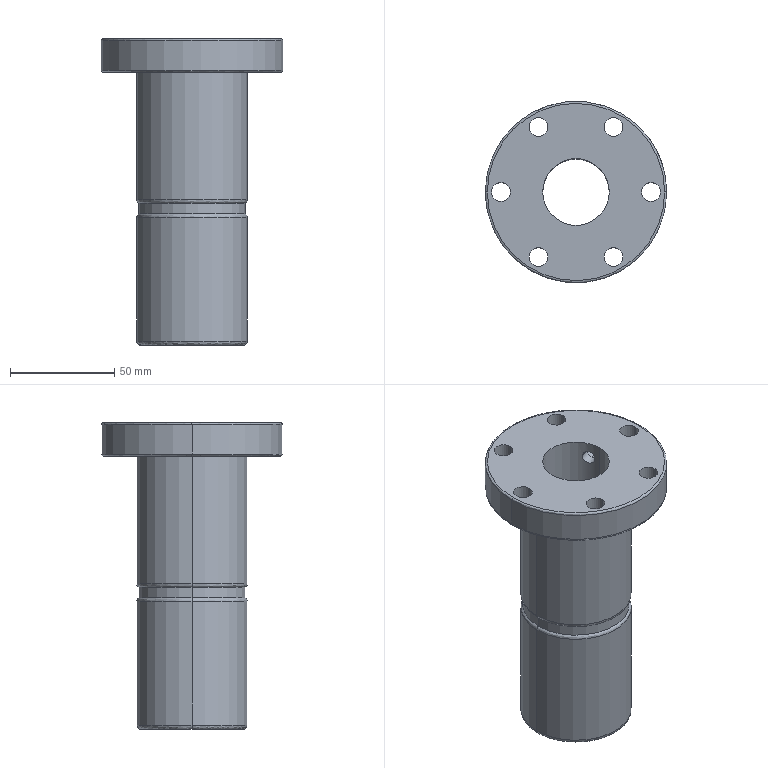Part | STEP file | 45LFDDC Lead Screw Seat | 1 solid | 44 faces | box 87 x 87 x 147 mm | volume 256572 mm3 | cylinder 28 | spline 10 | plane 4 | cone 2 | commonest cylinder face diameters 9 x12 53 x4 6.5 x2 6.8 x2 32 x2 39.972 x2